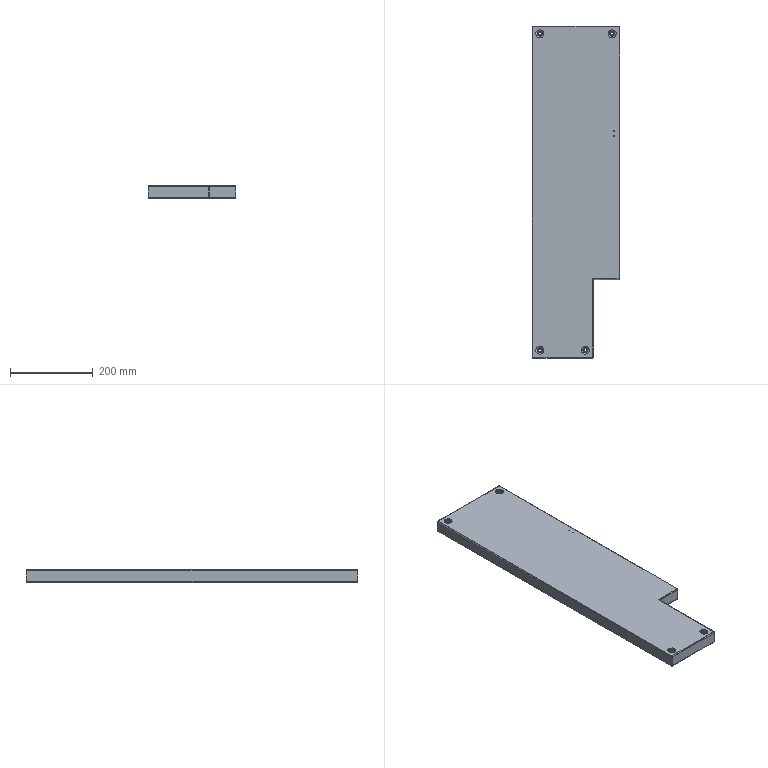Part | NX | 1 solid | 145 faces | box 213 x 804 x 30 mm | volume 355724 mm3 | plane 66 | cylinder 33 | spline 22 | torus 16 | cone 8 | commonest cylinder face diameters 1.473 x12 4.473 x12 2.5 x5 6.5 x4